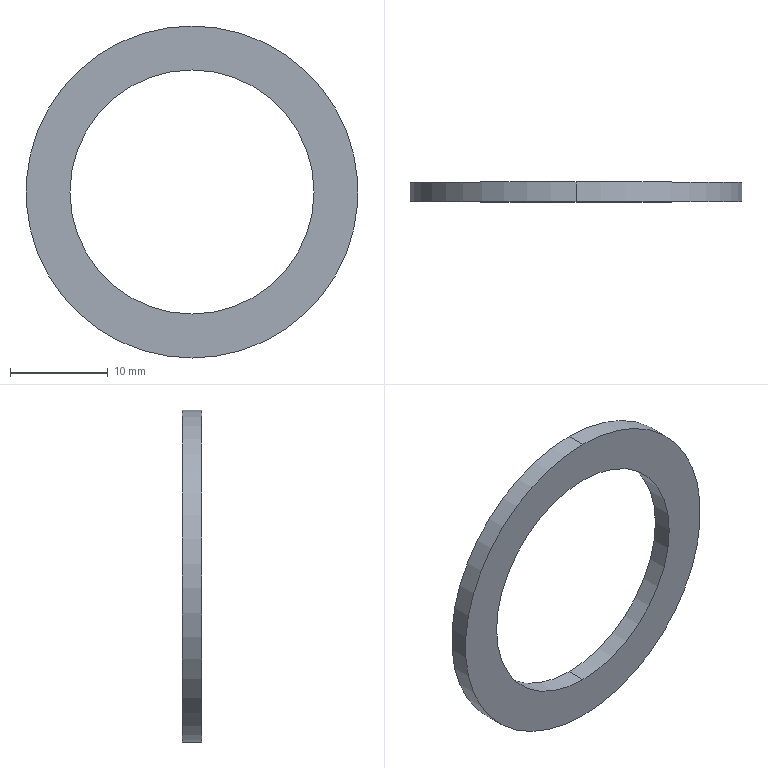Part | SolidWorks | features Extrusion 1 | 1 solid | 6 faces | box 34 x 2 x 34 mm | volume 834.093 mm3 | cylinder 4 | plane 2 | commonest cylinder face diameters 25 x2 34 x2
STEP:
#1=CARTESIAN_POINT('',(0.,1.,-12.5));
#2=VERTEX_POINT('',#1);
#3=CARTESIAN_POINT('',(0.,1.,12.5));
#4=VERTEX_POINT('',#3);
#5=CARTESIAN_POINT('',(0.,1.,0.));
#6=DIRECTION('',(0.,1.,0.));
#7=DIRECTION('',(0.,0.,1.));
#8=AXIS2_PLACEMENT_3D('',#5,#6,#7);
#9=CIRCLE('',#8,12.5);
#10=EDGE_CURVE('',#2,#4,#9,.T.);
#11=ORIENTED_EDGE('',*,*,#10,.T.);
#12=CARTESIAN_POINT('',(0.,-1.,12.5));
#13=VERTEX_POINT('',#12);
#14=CARTESIAN_POINT('',(0.,1.,12.5));
#15=DIRECTION('',(0.,-1.,0.));
#16=VECTOR('',#15,1000.);
#17=LINE('',#14,#16);
#18=EDGE_CURVE('',#4,#13,#17,.T.);
#19=ORIENTED_EDGE('',*,*,#18,.T.);
#20=CARTESIAN_POINT('',(0.,-1.,-12.5));
#21=VERTEX_POINT('',#20);
#22=CARTESIAN_POINT('',(0.,-1.,0.));
#23=DIRECTION('',(0.,1.,0.));
#24=DIRECTION('',(0.,0.,1.));
#25=AXIS2_PLACEMENT_3D('',#22,#23,#24);
#26=CIRCLE('',#25,12.5);
#27=EDGE_CURVE('',#21,#13,#26,.T.);
#28=ORIENTED_EDGE('',*,*,#27,.F.);
#29=CARTESIAN_POINT('',(0.,1.,-12.5));
#30=DIRECTION('',(0.,-1.,0.));
#31=VECTOR('',#30,1000.);
#32=LINE('',#29,#31);
#33=EDGE_CURVE('',#2,#21,#32,.T.);
#34=ORIENTED_EDGE('',*,*,#33,.F.);
#35=EDGE_LOOP('',(#11,#19,#28,#34));
#36=FACE_OUTER_BOUND('',#35,.T.);
#37=CARTESIAN_POINT('',(0.,1.,0.));
#38=DIRECTION('',(0.,-1.,0.));
#39=DIRECTION('',(0.,0.,-1.));
#40=AXIS2_PLACEMENT_3D('',#37,#38,#39);
#41=CYLINDRICAL_SURFACE('',#40,12.5);
#42=ADVANCED_FACE('',(#36),#41,.F.);
#43=CARTESIAN_POINT('',(0.,1.,17.));
#44=VERTEX_POINT('',#43);
#45=CARTESIAN_POINT('',(0.,1.,-17.));
#46=VERTEX_POINT('',#45);
#47=CARTESIAN_POINT('',(0.,1.,0.));
#48=DIRECTION('',(0.,1.,0.));
#49=DIRECTION('',(0.,0.,1.));
#50=AXIS2_PLACEMENT_3D('',#47,#48,#49);
#51=CIRCLE('',#50,17.);
#52=EDGE_CURVE('',#44,#46,#51,.T.);
#53=ORIENTED_EDGE('',*,*,#52,.F.);
#54=CARTESIAN_POINT('',(0.,-1.,17.));
#55=VERTEX_POINT('',#54);
#56=CARTESIAN_POINT('',(0.,1.,17.));
#57=DIRECTION('',(0.,-1.,0.));
#58=VECTOR('',#57,1000.);
#59=LINE('',#56,#58);
#60=EDGE_CURVE('',#44,#55,#59,.T.);
#61=ORIENTED_EDGE('',*,*,#60,.T.);
#62=CARTESIAN_POINT('',(0.,-1.,-17.));
#63=VERTEX_POINT('',#62);
#64=CARTESIAN_POINT('',(0.,-1.,0.));
#65=DIRECTION('',(0.,1.,0.));
#66=DIRECTION('',(0.,0.,1.));
#67=AXIS2_PLACEMENT_3D('',#64,#65,#66);
#68=CIRCLE('',#67,17.);
#69=EDGE_CURVE('',#55,#63,#68,.T.);
#70=ORIENTED_EDGE('',*,*,#69,.T.);
#71=CARTESIAN_POINT('',(0.,1.,-17.));
#72=DIRECTION('',(0.,-1.,0.));
#73=VECTOR('',#72,1000.);
#74=LINE('',#71,#73);
#75=EDGE_CURVE('',#46,#63,#74,.T.);
#76=ORIENTED_EDGE('',*,*,#75,.F.);
#77=EDGE_LOOP('',(#53,#61,#70,#76));
#78=FACE_OUTER_BOUND('',#77,.T.);
#79=CARTESIAN_POINT('',(0.,1.,0.));
#80=DIRECTION('',(0.,-1.,0.));
#81=DIRECTION('',(0.,0.,-1.));
#82=AXIS2_PLACEMENT_3D('',#79,#80,#81);
#83=CYLINDRICAL_SURFACE('',#82,17.);
#84=ADVANCED_FACE('',(#78),#83,.T.);
#85=CARTESIAN_POINT('',(0.,1.,0.));
#86=DIRECTION('',(0.,1.,0.));
#87=DIRECTION('',(0.,0.,1.));
#88=AXIS2_PLACEMENT_3D('',#85,#86,#87);
#89=CIRCLE('',#88,17.);
#90=EDGE_CURVE('',#46,#44,#89,.T.);
#91=ORIENTED_EDGE('',*,*,#90,.T.);
#92=ORIENTED_EDGE('',*,*,#52,.T.);
#93=EDGE_LOOP('',(#91,#92));
#94=FACE_OUTER_BOUND('',#93,.T.);
#95=ORIENTED_EDGE('',*,*,#10,.F.);
#96=CARTESIAN_POINT('',(0.,1.,0.));
#97=DIRECTION('',(0.,1.,0.));
#98=DIRECTION('',(0.,0.,1.));
#99=AXIS2_PLACEMENT_3D('',#96,#97,#98);
#100=CIRCLE('',#99,12.5);
#101=EDGE_CURVE('',#4,#2,#100,.T.);
#102=ORIENTED_EDGE('',*,*,#101,.F.);
#103=EDGE_LOOP('',(#95,#102));
#104=FACE_BOUND('',#103,.T.);
#105=CARTESIAN_POINT('',(0.,1.,0.));
#106=DIRECTION('',(0.,1.,0.));
#107=DIRECTION('',(0.,0.,1.));
#108=AXIS2_PLACEMENT_3D('',#105,#106,#107);
#109=PLANE('',#108);
#110=ADVANCED_FACE('',(#94,#104),#109,.T.);
#111=CARTESIAN_POINT('',(0.,-1.,0.));
#112=DIRECTION('',(0.,1.,0.));
#113=DIRECTION('',(0.,0.,1.));
#114=AXIS2_PLACEMENT_3D('',#111,#112,#113);
#115=CIRCLE('',#114,17.);
#116=EDGE_CURVE('',#63,#55,#115,.T.);
#117=ORIENTED_EDGE('',*,*,#116,.F.);
#118=ORIENTED_EDGE('',*,*,#69,.F.);
#119=EDGE_LOOP('',(#117,#118));
#120=FACE_OUTER_BOUND('',#119,.T.);
#121=ORIENTED_EDGE('',*,*,#27,.T.);
#122=CARTESIAN_POINT('',(0.,-1.,0.));
#123=DIRECTION('',(0.,1.,0.));
#124=DIRECTION('',(0.,0.,1.));
#125=AXIS2_PLACEMENT_3D('',#122,#123,#124);
#126=CIRCLE('',#125,12.5);
#127=EDGE_CURVE('',#13,#21,#126,.T.);
#128=ORIENTED_EDGE('',*,*,#127,.T.);
#129=EDGE_LOOP('',(#121,#128));
#130=FACE_BOUND('',#129,.T.);
#131=CARTESIAN_POINT('',(0.,-1.,0.));
#132=DIRECTION('',(0.,1.,0.));
#133=DIRECTION('',(0.,0.,1.));
#134=AXIS2_PLACEMENT_3D('',#131,#132,#133);
#135=PLANE('',#134);
#136=ADVANCED_FACE('',(#120,#130),#135,.F.);
#137=ORIENTED_EDGE('',*,*,#60,.F.);
#138=ORIENTED_EDGE('',*,*,#90,.F.);
#139=ORIENTED_EDGE('',*,*,#75,.T.);
#140=ORIENTED_EDGE('',*,*,#116,.T.);
#141=EDGE_LOOP('',(#137,#138,#139,#140));
#142=FACE_OUTER_BOUND('',#141,.T.);
#143=CARTESIAN_POINT('',(0.,1.,0.));
#144=DIRECTION('',(0.,-1.,0.));
#145=DIRECTION('',(0.,0.,-1.));
#146=AXIS2_PLACEMENT_3D('',#143,#144,#145);
#147=CYLINDRICAL_SURFACE('',#146,17.);
#148=ADVANCED_FACE('',(#142),#147,.T.);
#149=ORIENTED_EDGE('',*,*,#18,.F.);
#150=ORIENTED_EDGE('',*,*,#101,.T.);
#151=ORIENTED_EDGE('',*,*,#33,.T.);
#152=ORIENTED_EDGE('',*,*,#127,.F.);
#153=EDGE_LOOP('',(#149,#150,#151,#152));
#154=FACE_OUTER_BOUND('',#153,.T.);
#155=CARTESIAN_POINT('',(0.,1.,0.));
#156=DIRECTION('',(0.,-1.,0.));
#157=DIRECTION('',(0.,0.,-1.));
#158=AXIS2_PLACEMENT_3D('',#155,#156,#157);
#159=CYLINDRICAL_SURFACE('',#158,12.5);
#160=ADVANCED_FACE('',(#154),#159,.F.);
#161=CLOSED_SHELL('',(#42,#84,#110,#136,#148,#160));
#162=MANIFOLD_SOLID_BREP('',#161);
#163=CARTESIAN_POINT('',(0.,0.,0.));
#164=DIRECTION('',(0.,0.,1.));
#165=DIRECTION('',(1.,0.,0.));
#166=AXIS2_PLACEMENT_3D('',#163,#164,#165);
#167=(LENGTH_UNIT()NAMED_UNIT(*)SI_UNIT(.MILLI.,.METRE.));
#168=UNCERTAINTY_MEASURE_WITH_UNIT(LENGTH_MEASURE(0.00001),#167,'','');
#169=(NAMED_UNIT(*)PLANE_ANGLE_UNIT()SI_UNIT($,.RADIAN.));
#170=(NAMED_UNIT(*)SI_UNIT($,.STERADIAN.)SOLID_ANGLE_UNIT());
#171=(GEOMETRIC_REPRESENTATION_CONTEXT(3)GLOBAL_UNCERTAINTY_ASSIGNED_CONTEXT((#168))GLOBAL_UNIT_ASSIGNED_CONTEXT((#167,#169,#170))REPRESENTATION_CONTEXT('',''));
#172=ADVANCED_BREP_SHAPE_REPRESENTATION('',(#162,#166),#171);